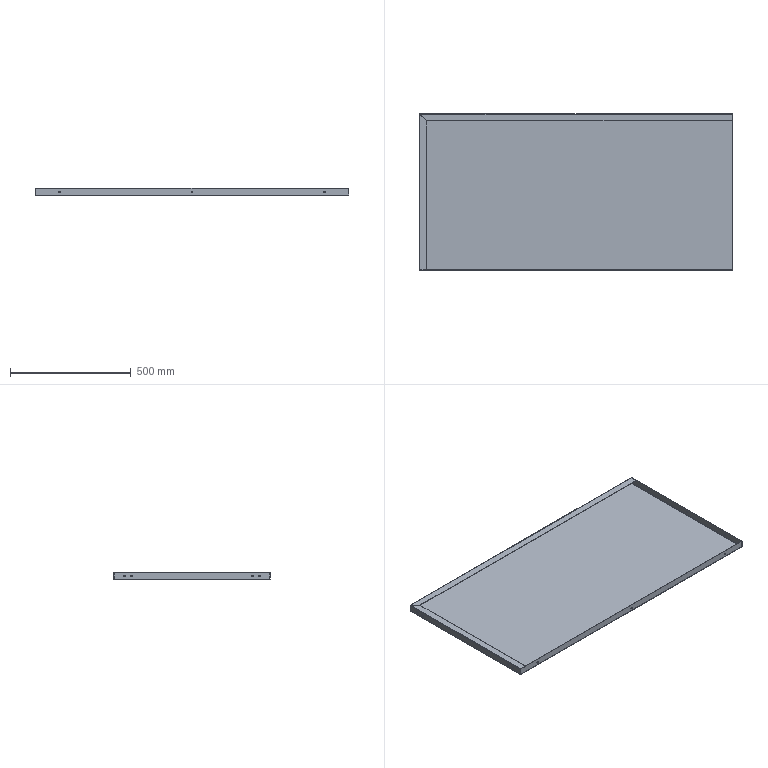Part | STEP file | Inner sheet metal 1 | 1 solid | 80 faces | box 1300 x 650 x 30 mm | volume 1507890 mm3 | cylinder 38 | plane 32 | spline 10 | commonest cylinder face diameters 7 x26 2 x6 5 x6